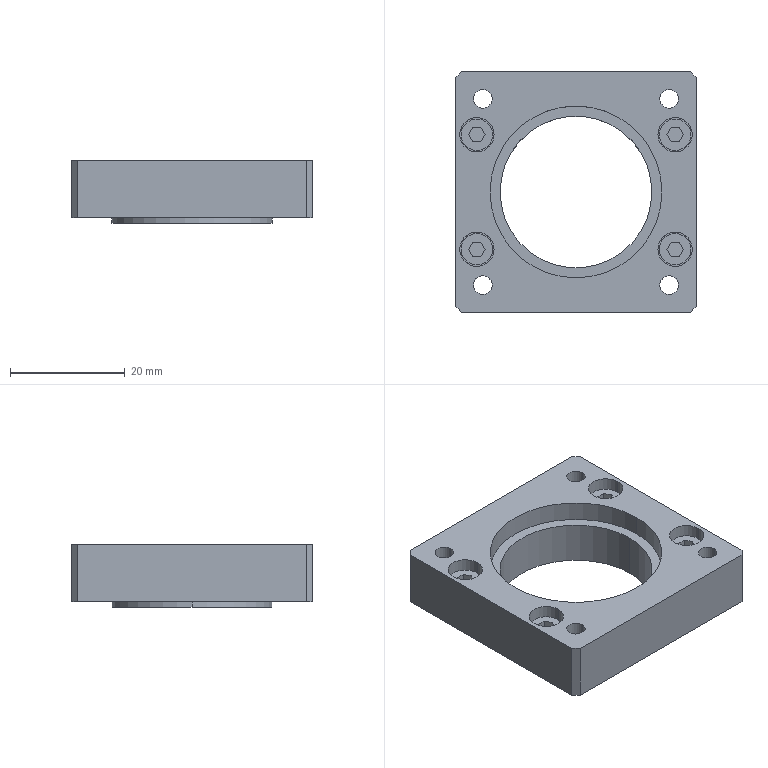Part | SolidWorks | features BaseBody 1 | 1 solid | 78 faces | box 42 x 42 x 11 mm | volume 10971 mm3 | plane 48 | cylinder 30 | commonest cylinder face diameters 3.242 x8 5.5 x8 6 x8 26.5 x2 28 x2 30 x2